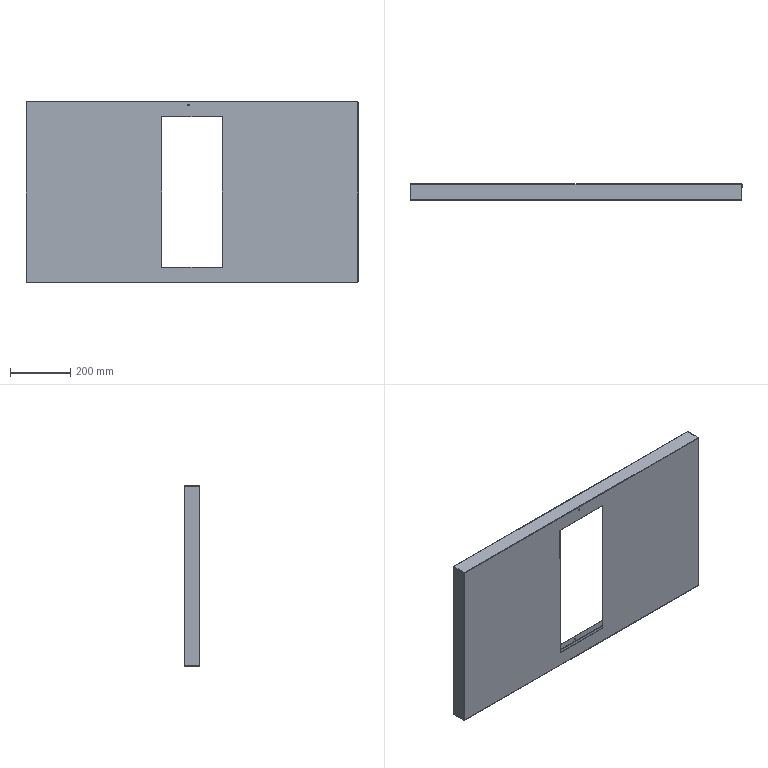Part | SolidWorks | features SplitBody 1 | 1 solid | 176 faces | box 1100 x 53 x 600.001 mm | volume 1427839 mm3 | plane 106 | cylinder 46 | spline 24 | commonest cylinder face diameters 0.2 x16 3.2 x16 3.5 x12 4.5 x2